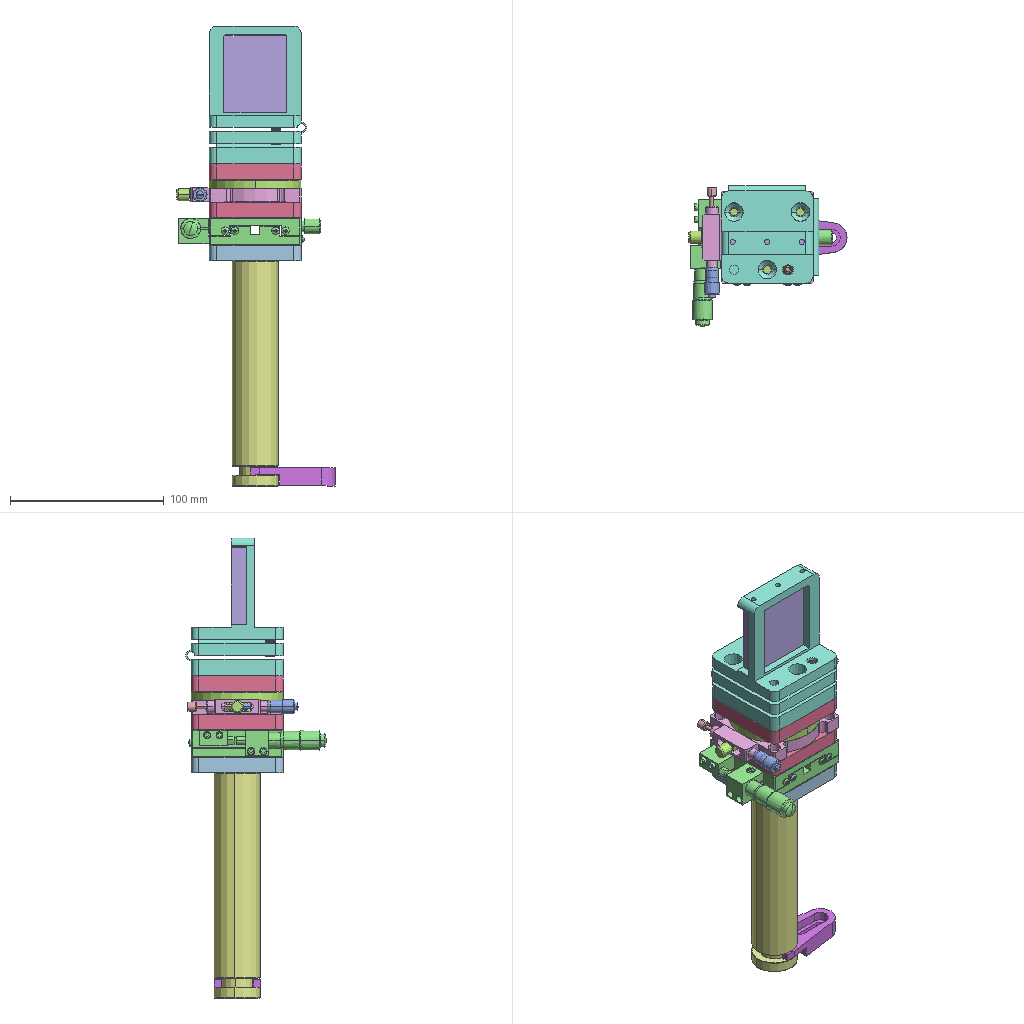Assembly | SolidWorks | 18 different items | 19 placed | box 103 x 91 x 299 mm
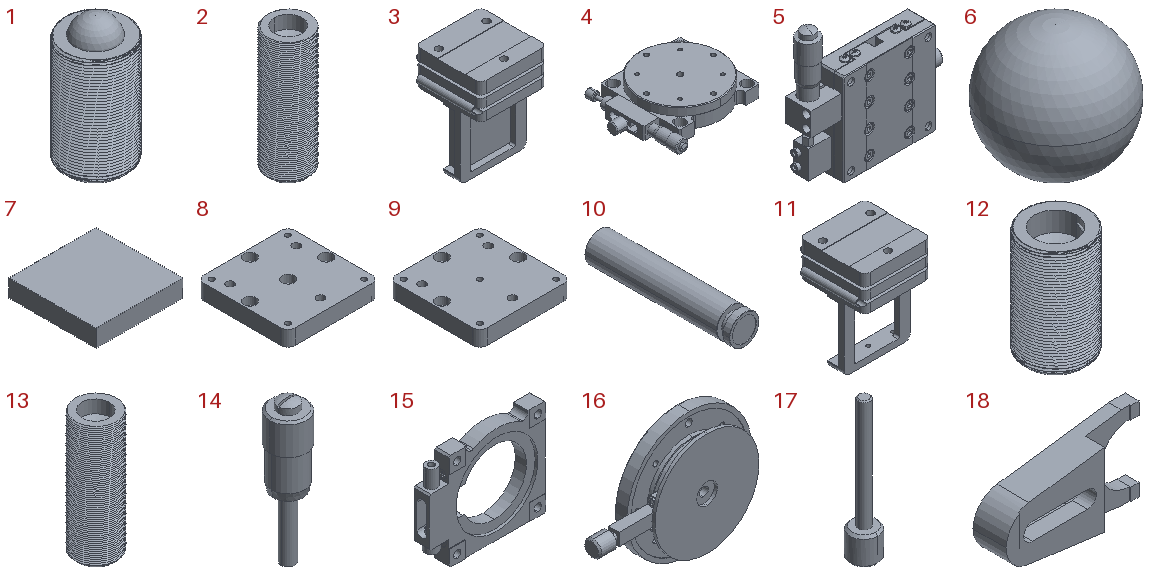Parts list (item | name | quantity | parent item | size | volume | features):
1 | (subassembly) | x1 | in 3 | 6.183 x 6.183 x 12.162 mm | 269.276 mm3 | -
2 | (subassembly) | x1 | in 3 | 6.183 x 6.183 x 18 mm | 451.29 mm3 | features RefAxis 1
3 | (subassembly) | x1 | - | 63.5 x 63.5 x 89.7 mm | 124553 mm3 | features CompositeCurve 1
4 | (subassembly) | x1 | - | 81 x 72.197 x 15 mm | 47712 mm3 | -
5 | - | x1 | - | 92.6 x 18 x 89.45 mm | 68470 mm3 | features BaseBody 1
6 | - | x1 | in 1 | 4 x 4 x 4 mm | 33.51 mm3 | features Revolution 1
7 | - | x1 | in 3 | 50 x 50 x 10 mm | 25000 mm3 | features Extrusion 1
8 | - | x1 | - | 60 x 60 x 10 mm | 33572 mm3 | features Cut 3, HoleWzd 3, Extrusion 1, Fillet 1, ICE 1
9 | - | x2 | - | 60 x 60 x 10 mm | 33807 mm3 | features HoleWzd 3, Cut 1, Extrusion 1, Fillet 1, ICE 1
10 | - | x1 | - | 30 x 146.6 x 30 mm | 100846 mm3 | features ICE 2, Chamfer 1, HoleWzd 1, MoveCopyBody 1, MoveFace 1, RefAxis 1, Revolution 1
11 | - | x1 | in 3 | 63.5 x 63.5 x 89.7 mm | 98956 mm3 | features ICE 23, HoleWzd 2, DelFace 1, Extrusion 1, Fillet 1
12 | - | x1 | in 1 | 6.183 x 6.183 x 10.5 mm | 236.179 mm3 | features ICE 5, RevCut 4, Extrusion 1, Fillet 1, Helix 1, RefAxis 1, Sweep 1
13 | - | x1 | in 2 | 6.183 x 6.183 x 18 mm | 451.29 mm3 | features ICE 3, RevCut 3, Extrusion 1, Fillet 1, Helix 1, RefAxis 1, Sweep 1
14 | - | x1 | in 4 | 9.3 x 9.3 x 36.697 mm | 794.178 mm3 | features BaseBody 1
15 | - | x1 | in 4 | 72 x 9.75 x 60 mm | 18365 mm3 | features BaseBody 1
16 | - | x1 | in 4 | 81 x 14.5 x 60 mm | 28270 mm3 | features BaseBody 1
17 | - | x1 | in 4 | 6 x 6 x 30 mm | 282.776 mm3 | features BaseBody 1
18 | - | x1 | - | 54.997 x 12 x 30 mm | 7361 mm3 | features ICE 4, Extrusion 1, Fillet 1
Mates (type | each side: item.copy, entity, surface, feature):
In the top assembly
Concentric | 10.1 face cylinder Revolve1 | 18.1 face cylinder Cut-Extrude2
Coincident | 10.1 face plane Revolve1 | 18.1 face plane Boss-Extrude1
Coincident | 16.1 face plane Input1 | 9.1 face plane Boss-Extrude1
Concentric | 16.1 face cylinder Input1 | 9.1 face cylinder Cut-Extrude2 | 2 times
In subassembly 3
Concentric | 11.1 face cylinder Cut-Extrude9 | 13.1 edge
Coincident | 11.1 face plane Cut-Extrude24 | 7.1 face plane Boss-Extrude1 | 2 times
Tangent | 11.1 face plane Boss-Extrude3 | 3.1 face
In subassembly 2
Coincident | 13.2 plane | 2.1 plane | 2 times
In subassembly 1
Tangent | 12.1 face cone Cut-Revolve3 | 6.1 face sphere Revolve1
Tangent | 12.1 face cylinder Cut-Revolve3 | 6.1 face sphere Revolve1